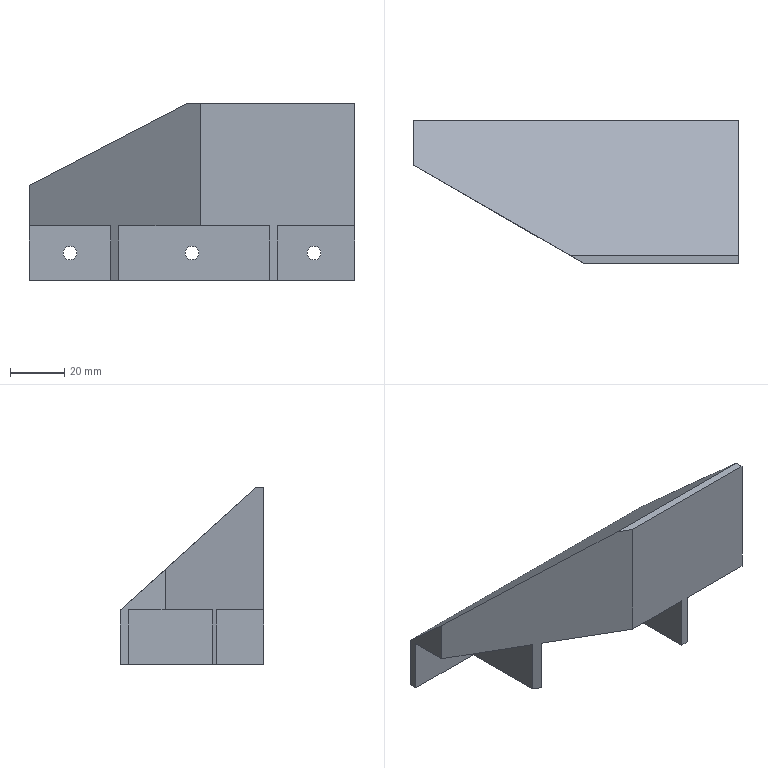Part | STEP file | Top plate | 1 solid | 29 faces | box 120 x 53 x 65 mm | volume 56002 mm3 | plane 23 | cylinder 6 | commonest cylinder face diameters 5.1 x6